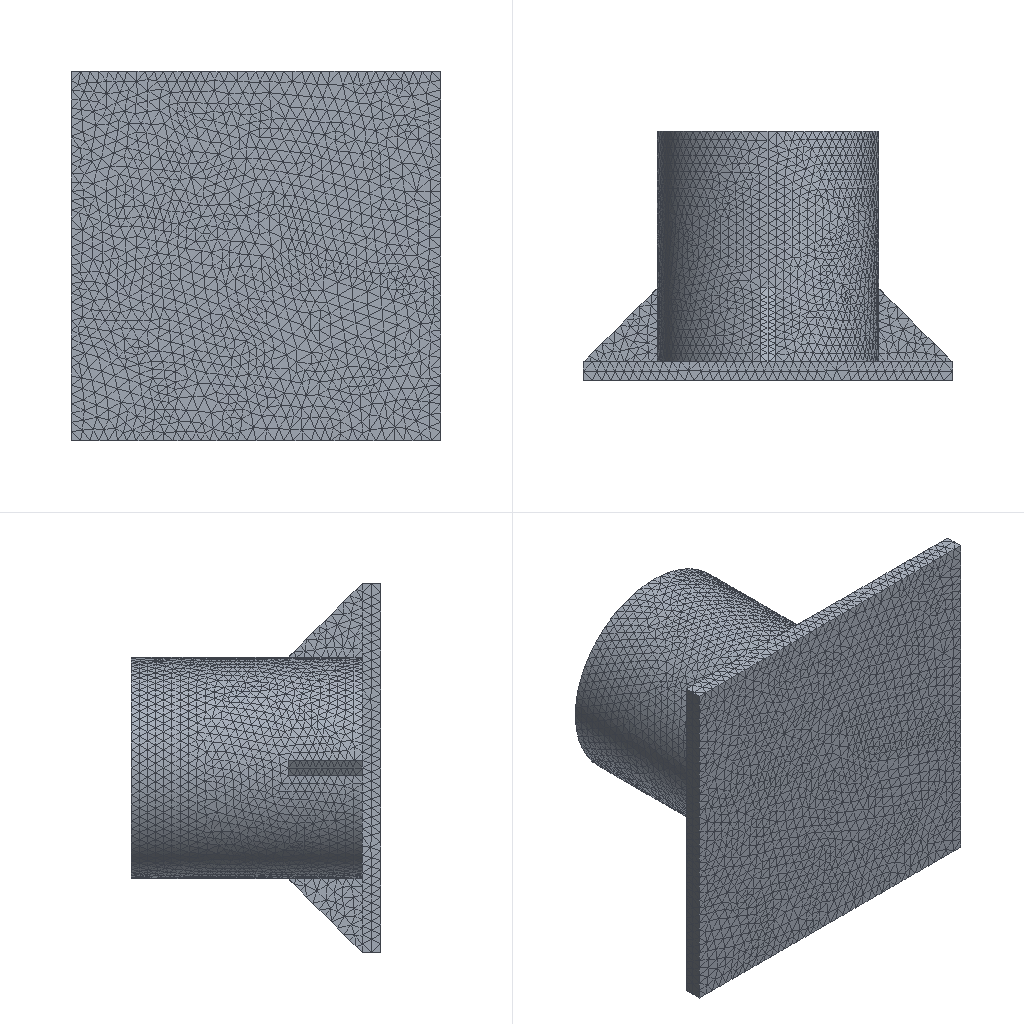Simulation study | ansys workbench
Set-up summary:
category,name,step,type,value,unit,region
solver,ansys_workbench
units,mm-N-s-tonne (MPa),,stated,"/units,MPA"
analysis,LS1,,static
load_step,LS1,LS1,static,nsubst=1; time=1
mesh,nodes,,,70250
mesh,elements,,,46024
element_type,SOLID187,,,41872
element_type,SURF154,,,3512
element_type,CONTA174,,,640
material,Structural Steel,,E,200000,tonne s^-2 mm^-1
material,Structural Steel,,nu,0.3
material,Structural Steel,,density,7.8e-09,tonne mm^-3
load,Define Pressure Using Surface Effect Elements,LS1,pressure,0.8,,SURF154 #10
bc,,LS1,fixed,"[dofs=ROTX,ROTY,ROTZ,UX,UY,UZ n=20]",,node list
contact,contact 1,,bonded (always),element=CONTA174
contact,contact 2,,bonded (always),element=CONTA174
contact,contact 3,,bonded (always),element=CONTA174
contact,contact 4,,bonded (always),element=CONTA174
named_set,REMOTEDISPALL,,node,4
Ansys APDL input file, long lists of numbers shortened:
/batch
/config,noeldb,1     ! force off writing results to database
*get,_wallstrt,active,,time,wall
! ANSYS input file written by Workbench version 2021 R1
! File used for geometry attach:
/title,wbnew--____ (B5)
! ****** Begin Custom Load Command Snippet ******
/COM, ACT Extensions:
/COM,     LSDYNA, 2021.1
/COM,
! ****** End   Custom Load Command Snippet ******
*DIM,_wb_ProjectScratch_dir,string,248
_wb_ProjectScratch_dir(1) = ''
*DIM,_wb_SolverFiles_dir,string,248
_wb_SolverFiles_dir(1) = ''
*DIM,_wb_userfiles_dir,string,248
_wb_userfiles_dir(1) = ''
/com,--- Data in consistent NMM units. See Solving Units in the help system for more information.
/units,MPA
/nopr
/wb,file,start              !  signify a WB generated input file
/prep7
! Turn off shape checking because checks already performed inside WB mesher.
! See help system for more information.
SHPP,OFF,,NOWARN
/nolist
etcon,set             ! allow ANSYS to choose best KEYOP's for 180x elements, resets any applicable keyopt to MAPDL defaults
/com,*********** Nodes for the whole assembly ***********
nblock,3,,77270
(1i9,3e20.9e3)
        1     0.000000000E+00     2.700000000E+03    -1.000000000E+03
! (70245 more lines like these left out)
-1
/com,*********** Nodes for all Remote Points ***********
nblock,3
(1i9,3e20.9e3)
    70247    -2.000000000E+03     1.000000000E+02    -3.725290298E-14
    70248    -2.000000000E+03     1.000000000E+02    -3.725290298E-14
    70249    -2.000000000E+03     1.000000000E+02    -3.725290298E-14
    70250    -2.000000000E+03     1.000000000E+02    -3.725290298E-14
-1
/wb,elem,start            !  set before creation of elements
/com,*********** Elements for Body 1 "__-FreeParts|____(____)1" ***********
et,1,187
eblock,19,solid,,41872
(19i9)
        1        1        1        1        0        0        0        0       10        0        1     8226    10631     9051     9803    64966    68065    64961    64962
! (83743 more lines like these left out)
-1
/wb,elem,end               !  done creating elements
/com,*********** Send User Defined Coordinate System(s) ***********
csys,0
toffst,273.15,  ! Temperature offset from absolute zero
/com,*********** Set Reference Temperature ***********
tref,22.
/wb,mat,start              !  starting to send materials
/com,*********** Send Materials ***********
MP,DENS,1,7.8e-09,	! tonne mm^-3
MP,EX,1,200000,	! tonne s^-2 mm^-1
MP,NUXY,1,0.3,
/wb,mat,end                !  done sending materials
!************************* Model Summary ********************
!__-FreeParts|____(____)1,	结构钢,	matid,	1
!************************* End Model Summary ********************
! get the diagonal of the bounding box. Needed later for other things
*get,_xmin,node,,mnloc,x
*get,_ymin,node,,mnloc,y
*get,_zmin,node,,mnloc,z
*get,_xmax,node,,mxloc,x
*get,_ymax,node,,mxloc,y
*get,_zmax,node,,mxloc,z
_ASMDIAG=(_xmax-_xmin)*(_xmax-_xmin)+(_ymax-_ymin)*(_ymax-_ymin)+(_zmax-_zmin)*(_zmax-_zmin)
_ASMDIAG=SQRT(_ASMDIAG)
/wb,contact,start          !  starting to send contact
/wb,contact,end            !  done creating contacts
/golist
/wb,load,start             !  starting to send loads
/com,*********** Create Remote Point "内部远程点" ***********
! -------- Remote Point Used by "远程位移" --------
*set,tid,3
*set,cid,2
et,cid,174
et,tid,170
keyo,tid,2,1               ! Don't fix the pilot node
keyo,tid,4,111111
keyo,cid,12,5              ! Bonded Contact
keyo,cid,4,1               ! Deformable RBE3 style load
keyo,cid,2,2               ! MPC style contact
eblock,10,,,160
(15i9)
    56103        2        2        2        0      538      561     4608     4608    14920    15056     4608    14922
! (159 more lines like these left out)
-1
*set,_npilot,70247
_npilot30=_npilot
type,tid
mat ,cid
real,cid
tshape,pilo
en,56263,_npilot
tshape
/com,*********** Create Remote Point "内部远程点" ***********
! -------- Remote Point Used by "远程位移 2" --------
*set,tid,5
*set,cid,4
et,cid,174
et,tid,170
keyo,tid,2,1               ! Don't fix the pilot node
keyo,tid,4,111111
keyo,cid,12,5              ! Bonded Contact
keyo,cid,4,1               ! Deformable RBE3 style load
keyo,cid,2,2               ! MPC style contact
eblock,10,,,160
(15i9)
    56264        4        4        4        0      379     4570      380      380    13806    13810      380    13803
! (159 more lines like these left out)
-1
*set,_npilot,70248
_npilot33=_npilot
type,tid
mat ,cid
real,cid
tshape,pilo
en,56424,_npilot
tshape
/com,*********** Create Remote Point "内部远程点" ***********
! -------- Remote Point Used by "远程位移 3" --------
*set,tid,7
*set,cid,6
et,cid,174
et,tid,170
keyo,tid,2,1               ! Don't fix the pilot node
keyo,tid,4,111111
keyo,cid,12,5              ! Bonded Contact
keyo,cid,4,1               ! Deformable RBE3 style load
keyo,cid,2,2               ! MPC style contact
eblock,10,,,160
(15i9)
    56425        6        6        6        0      455      456     4685     4685    14423    14430     4685    14426
! (159 more lines like these left out)
-1
*set,_npilot,70249
_npilot36=_npilot
type,tid
mat ,cid
real,cid
tshape,pilo
en,56585,_npilot
tshape
/com,*********** Create Remote Point "内部远程点" ***********
! -------- Remote Point Used by "远程位移 4" --------
*set,tid,9
*set,cid,8
et,cid,174
et,tid,170
keyo,tid,2,1               ! Don't fix the pilot node
keyo,tid,4,111111
keyo,cid,12,5              ! Bonded Contact
keyo,cid,4,1               ! Deformable RBE3 style load
keyo,cid,2,2               ! MPC style contact
eblock,10,,,160
(15i9)
    56586        8        8        8        0      264     4645      559      559    12988    15049      559    12986
! (159 more lines like these left out)
-1
*set,_npilot,70250
_npilot39=_npilot
type,tid
mat ,cid
real,cid
tshape,pilo
en,56746,_npilot
tshape
/com,*********** Define Pressure Using Surface Effect Elements ***********
et,10,154
eblock,10,,,3512
(15i9)
    56747       10       10       10        0       15       16     3719     3719    10714    10722     3719    10716
! (3511 more lines like these left out)
-1
esel,s,type,,10
keyop,10,7,0                ! Use deformed area for application of load
esel,all
/com,*********** Construct Remote Displacement ***********
/com,*********** Construct Remote Displacement ***********
/com,*********** Construct Remote Displacement ***********
/com,*********** Construct Remote Displacement ***********
/COM,*** Create a component for all remote displacements ***
CMBLOCK,REMOTEDISPALL,NODE,        4
(8i10)
     70247     70248     70249     70250
esel,all
/gst,on,on
fini
*get,_numnode,node,0,count
*get,_numelem,elem,0,count
*get, _MAXELEMNUM, elem, 0, NUM, MAX
*get, _MAXNODENUM, node, 0, NUM, MAX
*get, _MAXELEMTYPE, etyp, 0, NUM, MAX
*get, _MAXREALCONST, real, 0, NUM, MAX
/go
/wb,load,end               !  done creating loads
/com,--- Number of total nodes = %_numnode%
/com,--- Number of contact elements = 4152
/com,--- Number of spring elements = 0
/com,--- Number of bearing elements = 0
/com,--- Number of solid elements = 41872
/com,--- Number of condensed parts = 0
/com,--- Number of total elements = %_numelem%
*get,_wallbsol,active,,time,wall
/com,****************************************************************************
/com,*************************    SOLUTION       ********************************
/com,****************************************************************************
/solu
antype,0                   ! static analysis
_thickRatio=  1     ! Ratio of thick parts in the model
eqsl,pcg,1e-8,,,,,,1
cntr,print,1               ! print out contact info and also make no initial contact an error
dmpoption,emat,no             ! Don't combine emat file for DANSYS
dmpoption,esav,no             ! Don't combine esav file for DANSYS
nldiag,cont,iter           ! print out contact info each equilibrium iteration
rescontrol,,none                 ! Do not keep any restart files
/com,****************************************************
/com,******************* SOLVE FOR LS 1 OF 1 ****************
esel,s,type,,10
nsle
sf,all,pres,0.8
nsel,all
esel,all
d,70247,ux,0.
d,70247,uy,0.
d,70247,uz,0.
d,70247,rotx,0.
d,70247,roty,0.
d,70248,ux,0.
d,70248,uy,0.
d,70248,uz,0.
d,70248,roty,0.
d,70248,rotz,0.
d,70249,ux,0.
d,70249,uy,0.
d,70249,uz,0.
d,70249,rotx,0.
d,70249,roty,0.
d,70250,ux,0.
d,70250,uy,0.
d,70250,uz,0.
d,70250,roty,0.
d,70250,rotz,0.
esel,all
/nopr
/gopr
/nolist
nsub,1,1,1
time,1.
outres,erase
outres,all,none
outres,nsol,all,
outres,rsol,all
outres,eangl,all
outres,etmp,all
outres,veng,all
outres,strs,all,
outres,epel,all,
outres,eppl,all,
outres,cont,all,
! *********** WB SOLVE COMMAND ***********
! check interactive state
*get,ANSINTER_,active,,int
*if,ANSINTER_,ne,0,then
/eof
*endif
solve
/com *************** Write FE CONNECTORS *********
CEWRITE,file,ce,,INTE
/com,****************************************************
/com,*************** FINISHED SOLVE FOR LS 1 *************
*get,_wallasol,active,,time,wall
/nopr
*get,_numnode,node,0,count
*get,_numelem,elem,0,count
*get, _MAXELEMNUM, elem, 0, NUM, MAX
*get, _MAXNODENUM, node, 0, NUM, MAX,,,INTERNAL
*get, _MAXELEMTYPE, etyp, 0, NUM, MAX
*get, _MAXREALCONST, real, 0, NUM, MAX
/gopr
*get,_PCGITER,active,,solu,cgiter
/post1
xmlo,ENCODING,ISO-8859-1
xmlo,parm
/xml,parm,xml
fini
/gopr
*get,_walldone,active,,time,wall
_preptime=(_wallbsol-_wallstrt)*3600
_solvtime=(_wallasol-_wallbsol)*3600
_posttime=(_walldone-_wallasol)*3600
_totaltim=(_walldone-_wallstrt)*3600
*get,_dlbratio,active,0,solu,dlbr
*get,_combtime,active,0,solu,comb
/com,--- Total number of nodes = %_numnode%
/com,--- Total number of elements = %_numelem%
/com,--- Element load balance ratio = %_dlbratio%
/com,--- Time to combine distributed files = %_combtime%
/wb,file,end               ! done with WB generated input
Results summary:
result,analyses[0].index,,,1
result,analyses[0].system,,,SYS-1
result,analyses[0].deck,,,deck.dat
result,analyses[0].solve_status,,,completed
result,analyses[0].analysis_type,,,static
result,analyses[0].physics,,,mechanical
result,analyses[0].unit_system,,,"NMM: mm, ton, N, s, mV, mA, degC"
result,analyses[0].n_sets,,,1
result,analyses[0].load_steps[0].set,set=1,,1
result,analyses[0].load_steps[0].time_or_freq,set=1,,1
result,analyses[0].load_steps[0].max_displacement_magnitude,set=1,,0.04651
result,analyses[0].load_steps[0].max_von_mises_nodal,set=1,,5.438
result,analyses[0].load_steps[0].reaction_force_sum_xyz[1],set=1,,0.7193
result,analyses[0].load_steps[0].reaction_force_sum_xyz[2],set=1,,-0.4318
result,analyses[0].load_steps[0].reaction_force_sum_xyz[3],set=1,,-1.226
result,geometry_export[0][0],,,.step
result,geometry_export[0][1],,,ok
result,geometry_export[0][2],,,1